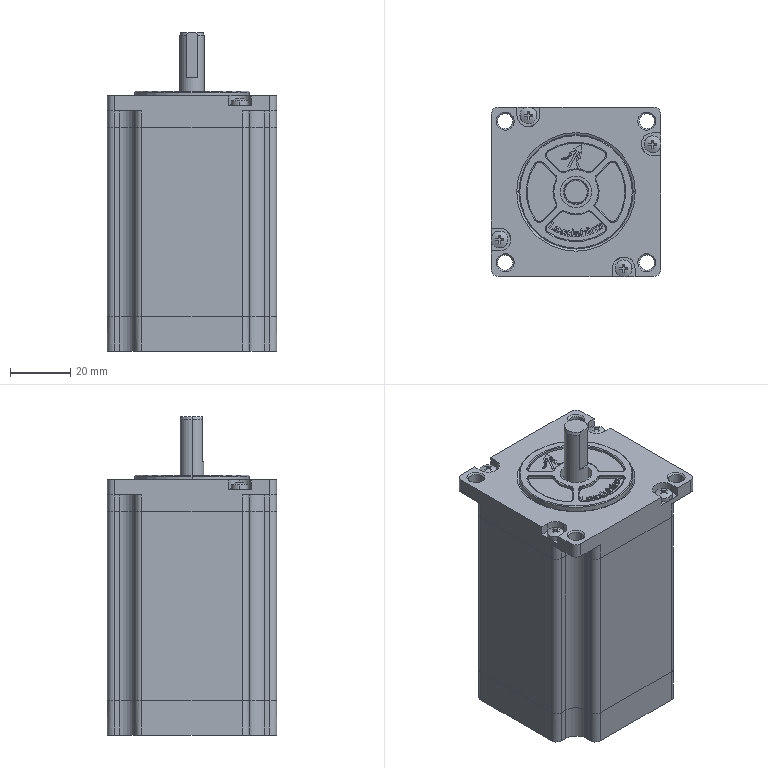Part | SolidWorks | 4 solids | 1485 faces | box 56.538 x 56.538 x 106 mm | volume 169179 mm3 | plane 967 | cylinder 270 | spline 207 | cone 41 | commonest cylinder face diameters 0.6 x62 3 x42 4.6 x28 2.7 x16 5.6 x16 10 x12